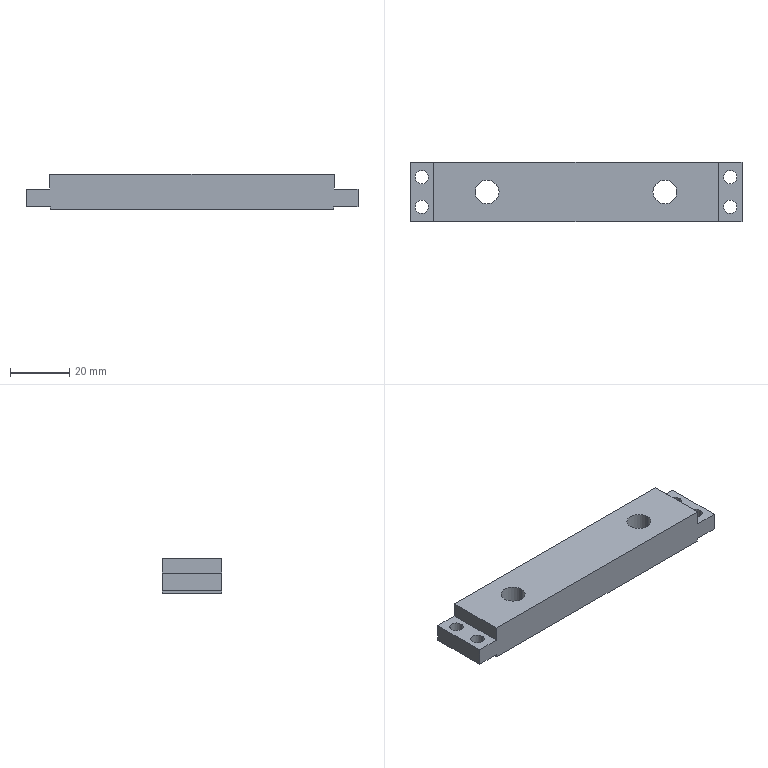Part | STEP file | 2054 Buffer mounting seat | 1 solid | 32 faces | box 112 x 20 x 12 mm | volume 23091 mm3 | cylinder 16 | plane 16 | commonest cylinder face diameters 4.5 x8 8.1 x4 12 x4